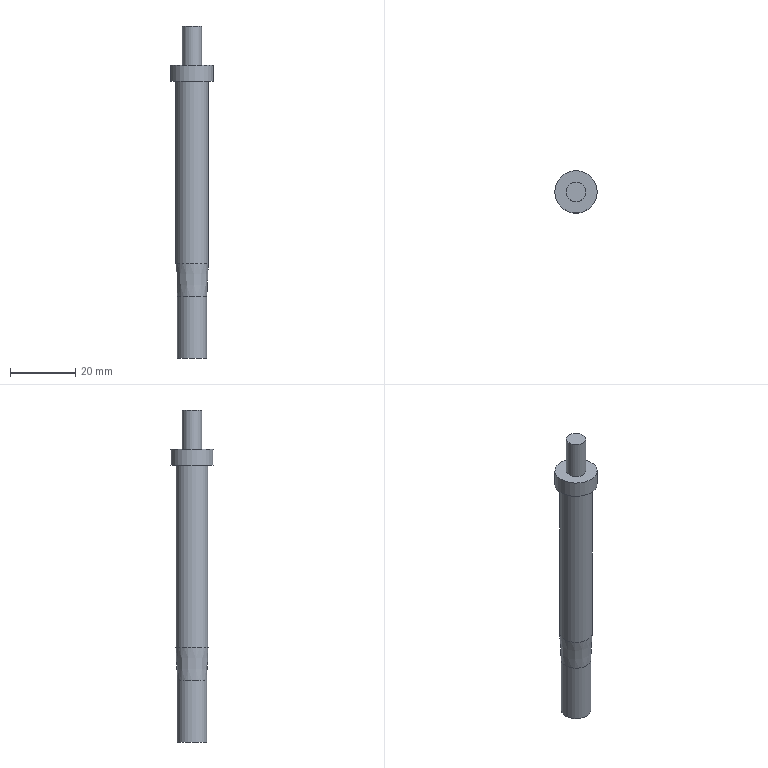Part | NX | features solid 2 | 1 solid | 9 faces | box 13 x 13 x 102 mm | volume 7354 mm3 | plane 4 | cylinder 4 | cone 1 | commonest cylinder face diameters 6 x1 9.1 x1 10 x1 13 x1
STEP:
#1=CARTESIAN_POINT('',(-511.046,-162.103,-16.));
#2=VERTEX_POINT('',#1);
#3=CARTESIAN_POINT('',(-515.596,-162.103,-16.));
#4=DIRECTION('',(0.,0.,1.));
#5=DIRECTION('',(1.,0.,0.));
#6=AXIS2_PLACEMENT_3D('',#3,#4,#5);
#7=CIRCLE('',#6,4.55);
#8=EDGE_CURVE('',#2,#2,#7,.T.);
#9=ORIENTED_EDGE('',*,*,#8,.F.);
#10=EDGE_LOOP('',(#9));
#11=FACE_BOUND('',#10,.T.);
#12=CARTESIAN_POINT('',(-515.596,-162.103,-16.));
#13=DIRECTION('',(0.,0.,-1.));
#14=DIRECTION('',(-1.,0.,0.));
#15=AXIS2_PLACEMENT_3D('',#12,#13,#14);
#16=PLANE('',#15);
#17=ADVANCED_FACE('',(#11),#16,.T.);
#18=CARTESIAN_POINT('',(-511.046,-162.103,3.));
#19=VERTEX_POINT('',#18);
#20=CARTESIAN_POINT('',(-515.596,-162.103,3.));
#21=DIRECTION('',(0.,0.,1.));
#22=DIRECTION('',(1.,0.,0.));
#23=AXIS2_PLACEMENT_3D('',#20,#21,#22);
#24=CIRCLE('',#23,4.55);
#25=EDGE_CURVE('',#19,#19,#24,.T.);
#26=ORIENTED_EDGE('',*,*,#25,.F.);
#27=EDGE_LOOP('',(#26));
#28=FACE_BOUND('',#27,.T.);
#29=ORIENTED_EDGE('',*,*,#8,.T.);
#30=EDGE_LOOP('',(#29));
#31=FACE_BOUND('',#30,.T.);
#32=CARTESIAN_POINT('',(-515.596,-162.103,-16.));
#33=DIRECTION('',(0.,0.,1.));
#34=DIRECTION('',(1.,0.,0.));
#35=AXIS2_PLACEMENT_3D('',#32,#33,#34);
#36=CYLINDRICAL_SURFACE('',#35,4.55);
#37=ADVANCED_FACE('',(#28,#31),#36,.T.);
#38=ORIENTED_EDGE('',*,*,#25,.T.);
#39=EDGE_LOOP('',(#38));
#40=FACE_BOUND('',#39,.T.);
#41=CARTESIAN_POINT('',(-510.596,-162.103,13.));
#42=VERTEX_POINT('',#41);
#43=CARTESIAN_POINT('',(-515.596,-162.103,13.));
#44=DIRECTION('',(0.,0.,1.));
#45=DIRECTION('',(1.,0.,0.));
#46=AXIS2_PLACEMENT_3D('',#43,#44,#45);
#47=CIRCLE('',#46,5.);
#48=EDGE_CURVE('',#42,#42,#47,.T.);
#49=ORIENTED_EDGE('',*,*,#48,.F.);
#50=EDGE_LOOP('',(#49));
#51=FACE_BOUND('',#50,.T.);
#52=CARTESIAN_POINT('',(-515.596,-162.103,3.));
#53=DIRECTION('',(0.,0.,1.));
#54=DIRECTION('',(1.,0.,0.));
#55=AXIS2_PLACEMENT_3D('',#52,#53,#54);
#56=CONICAL_SURFACE('',#55,4.55,0.04497);
#57=ADVANCED_FACE('',(#40,#51),#56,.T.);
#58=CARTESIAN_POINT('',(-520.596,-162.103,69.));
#59=VERTEX_POINT('',#58);
#60=CARTESIAN_POINT('',(-515.596,-162.103,69.));
#61=DIRECTION('',(0.,0.,-1.));
#62=DIRECTION('',(-1.,0.,0.));
#63=AXIS2_PLACEMENT_3D('',#60,#61,#62);
#64=CIRCLE('',#63,5.);
#65=EDGE_CURVE('',#59,#59,#64,.F.);
#66=ORIENTED_EDGE('',*,*,#65,.F.);
#67=EDGE_LOOP('',(#66));
#68=FACE_BOUND('',#67,.T.);
#69=ORIENTED_EDGE('',*,*,#48,.T.);
#70=EDGE_LOOP('',(#69));
#71=FACE_BOUND('',#70,.T.);
#72=CARTESIAN_POINT('',(-515.596,-162.103,13.));
#73=DIRECTION('',(0.,0.,1.));
#74=DIRECTION('',(1.,0.,0.));
#75=AXIS2_PLACEMENT_3D('',#72,#73,#74);
#76=CYLINDRICAL_SURFACE('',#75,5.);
#77=ADVANCED_FACE('',(#68,#71),#76,.T.);
#78=CARTESIAN_POINT('',(-512.596,-162.103,74.));
#79=VERTEX_POINT('',#78);
#80=CARTESIAN_POINT('',(-515.596,-162.103,74.));
#81=DIRECTION('',(0.,0.,1.));
#82=DIRECTION('',(1.,0.,0.));
#83=AXIS2_PLACEMENT_3D('',#80,#81,#82);
#84=CIRCLE('',#83,3.);
#85=EDGE_CURVE('',#79,#79,#84,.T.);
#86=ORIENTED_EDGE('',*,*,#85,.F.);
#87=EDGE_LOOP('',(#86));
#88=FACE_BOUND('',#87,.T.);
#89=CARTESIAN_POINT('',(-522.096,-162.103,74.));
#90=VERTEX_POINT('',#89);
#91=CARTESIAN_POINT('',(-515.596,-162.103,74.));
#92=DIRECTION('',(0.,0.,-1.));
#93=DIRECTION('',(-1.,0.,0.));
#94=AXIS2_PLACEMENT_3D('',#91,#92,#93);
#95=CIRCLE('',#94,6.5);
#96=EDGE_CURVE('',#90,#90,#95,.T.);
#97=ORIENTED_EDGE('',*,*,#96,.F.);
#98=EDGE_LOOP('',(#97));
#99=FACE_BOUND('',#98,.T.);
#100=CARTESIAN_POINT('',(-515.596,-162.103,74.));
#101=DIRECTION('',(0.,0.,1.));
#102=DIRECTION('',(1.,0.,0.));
#103=AXIS2_PLACEMENT_3D('',#100,#101,#102);
#104=PLANE('',#103);
#105=ADVANCED_FACE('',(#88,#99),#104,.T.);
#106=ORIENTED_EDGE('',*,*,#65,.T.);
#107=EDGE_LOOP('',(#106));
#108=FACE_BOUND('',#107,.T.);
#109=CARTESIAN_POINT('',(-509.096,-162.103,69.));
#110=VERTEX_POINT('',#109);
#111=CARTESIAN_POINT('',(-515.596,-162.103,69.));
#112=DIRECTION('',(0.,0.,1.));
#113=DIRECTION('',(1.,0.,0.));
#114=AXIS2_PLACEMENT_3D('',#111,#112,#113);
#115=CIRCLE('',#114,6.5);
#116=EDGE_CURVE('',#110,#110,#115,.T.);
#117=ORIENTED_EDGE('',*,*,#116,.F.);
#118=EDGE_LOOP('',(#117));
#119=FACE_BOUND('',#118,.T.);
#120=CARTESIAN_POINT('',(-515.596,-162.103,69.));
#121=DIRECTION('',(0.,0.,-1.));
#122=DIRECTION('',(-1.,0.,0.));
#123=AXIS2_PLACEMENT_3D('',#120,#121,#122);
#124=PLANE('',#123);
#125=ADVANCED_FACE('',(#108,#119),#124,.T.);
#126=ORIENTED_EDGE('',*,*,#96,.T.);
#127=EDGE_LOOP('',(#126));
#128=FACE_BOUND('',#127,.T.);
#129=ORIENTED_EDGE('',*,*,#116,.T.);
#130=EDGE_LOOP('',(#129));
#131=FACE_BOUND('',#130,.T.);
#132=CARTESIAN_POINT('',(-515.596,-162.103,69.));
#133=DIRECTION('',(0.,0.,1.));
#134=DIRECTION('',(1.,0.,0.));
#135=AXIS2_PLACEMENT_3D('',#132,#133,#134);
#136=CYLINDRICAL_SURFACE('',#135,6.5);
#137=ADVANCED_FACE('',(#128,#131),#136,.T.);
#138=CARTESIAN_POINT('',(-518.596,-162.103,86.));
#139=VERTEX_POINT('',#138);
#140=CARTESIAN_POINT('',(-515.596,-162.103,86.));
#141=DIRECTION('',(0.,0.,-1.));
#142=DIRECTION('',(-1.,0.,0.));
#143=AXIS2_PLACEMENT_3D('',#140,#141,#142);
#144=CIRCLE('',#143,3.);
#145=EDGE_CURVE('',#139,#139,#144,.T.);
#146=ORIENTED_EDGE('',*,*,#145,.F.);
#147=EDGE_LOOP('',(#146));
#148=FACE_BOUND('',#147,.T.);
#149=CARTESIAN_POINT('',(-515.596,-162.103,86.));
#150=DIRECTION('',(0.,0.,1.));
#151=DIRECTION('',(1.,0.,0.));
#152=AXIS2_PLACEMENT_3D('',#149,#150,#151);
#153=PLANE('',#152);
#154=ADVANCED_FACE('',(#148),#153,.T.);
#155=ORIENTED_EDGE('',*,*,#145,.T.);
#156=EDGE_LOOP('',(#155));
#157=FACE_BOUND('',#156,.T.);
#158=ORIENTED_EDGE('',*,*,#85,.T.);
#159=EDGE_LOOP('',(#158));
#160=FACE_BOUND('',#159,.T.);
#161=CARTESIAN_POINT('',(-515.596,-162.103,74.));
#162=DIRECTION('',(0.,0.,1.));
#163=DIRECTION('',(1.,0.,0.));
#164=AXIS2_PLACEMENT_3D('',#161,#162,#163);
#165=CYLINDRICAL_SURFACE('',#164,3.);
#166=ADVANCED_FACE('',(#157,#160),#165,.T.);
#167=CLOSED_SHELL('',(#17,#37,#57,#77,#105,#125,#137,#154,#166));
#168=MANIFOLD_SOLID_BREP('',#167);
#169=(LENGTH_UNIT()NAMED_UNIT(*)SI_UNIT(.MILLI.,.METRE.));
#170=UNCERTAINTY_MEASURE_WITH_UNIT(LENGTH_MEASURE(0.00001),#169,'','');
#171=(NAMED_UNIT(*)PLANE_ANGLE_UNIT()SI_UNIT($,.RADIAN.));
#172=(NAMED_UNIT(*)SI_UNIT($,.STERADIAN.)SOLID_ANGLE_UNIT());
#173=(GEOMETRIC_REPRESENTATION_CONTEXT(3)GLOBAL_UNCERTAINTY_ASSIGNED_CONTEXT((#170))GLOBAL_UNIT_ASSIGNED_CONTEXT((#169,#171,#172))REPRESENTATION_CONTEXT('',''));
#174=ADVANCED_BREP_SHAPE_REPRESENTATION('',(#168),#173);